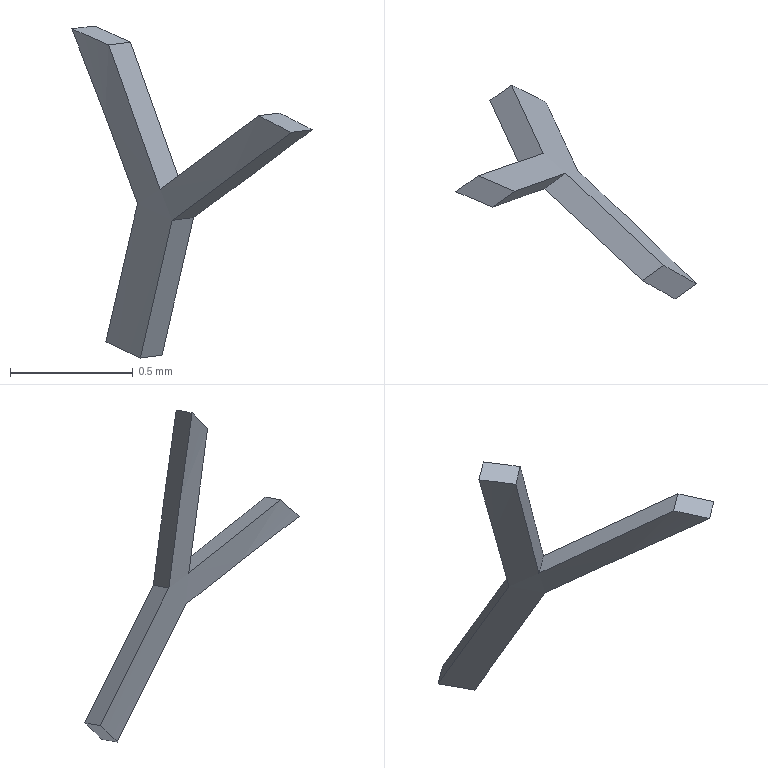Part | SolidWorks | features BaseBody 1 | 1 solid | 11 faces | box 0.9771 x 0.8707 x 1.35 mm | volume 0.03036 mm3 | plane 9 | cylinder 2 | commonest cylinder face diameters 16.8 x1 17 x1
STEP:
#1=CARTESIAN_POINT('',(1971.121,-237.195,995.991));
#2=VERTEX_POINT('',#1);
#3=CARTESIAN_POINT('',(1971.25,-237.473,996.551));
#4=VERTEX_POINT('',#3);
#5=CARTESIAN_POINT('',(1971.931,-238.948,999.517));
#6=DIRECTION('',(0.2015,-0.436,0.8771));
#7=VECTOR('',#6,1000.);
#8=LINE('',#5,#7);
#9=EDGE_CURVE('',#2,#4,#8,.T.);
#10=ORIENTED_EDGE('',*,*,#9,.T.);
#11=CARTESIAN_POINT('',(1971.734,-237.933,996.909));
#12=VERTEX_POINT('',#11);
#13=CARTESIAN_POINT('',(1971.25,-237.473,996.551));
#14=CARTESIAN_POINT('',(1971.414,-237.623,996.67));
#15=CARTESIAN_POINT('',(1971.575,-237.777,996.79));
#16=CARTESIAN_POINT('',(1971.734,-237.933,996.909));
#17=B_SPLINE_CURVE_WITH_KNOTS('',3,(#13,#14,#15,#16),.UNSPECIFIED.,.F.,.F.,(4,4),(0.,1.),.UNSPECIFIED.);
#18=EDGE_CURVE('',#4,#12,#17,.T.);
#19=ORIENTED_EDGE('',*,*,#18,.T.);
#20=CARTESIAN_POINT('',(1971.601,-237.859,996.976));
#21=VERTEX_POINT('',#20);
#22=CARTESIAN_POINT('',(1966.892,-244.458,994.777));
#23=DIRECTION('',(0.2015,-0.436,0.8771));
#24=DIRECTION('',(-0.7309,-0.6631,-0.1618));
#25=AXIS2_PLACEMENT_3D('',#22,#23,#24);
#26=CIRCLE('',#25,8.4);
#27=EDGE_CURVE('',#12,#21,#26,.T.);
#28=ORIENTED_EDGE('',*,*,#27,.T.);
#29=CARTESIAN_POINT('',(1971.201,-237.485,996.678));
#30=VERTEX_POINT('',#29);
#31=CARTESIAN_POINT('',(1971.201,-237.485,996.678));
#32=CARTESIAN_POINT('',(1971.336,-237.607,996.777));
#33=CARTESIAN_POINT('',(1971.47,-237.732,996.877));
#34=CARTESIAN_POINT('',(1971.601,-237.859,996.976));
#35=B_SPLINE_CURVE_WITH_KNOTS('',3,(#31,#32,#33,#34),.UNSPECIFIED.,.F.,.F.,(4,4),(0.,1.),.UNSPECIFIED.);
#36=EDGE_CURVE('',#30,#21,#35,.T.);
#37=ORIENTED_EDGE('',*,*,#36,.F.);
#38=CARTESIAN_POINT('',(1970.991,-237.561,997.264));
#39=VERTEX_POINT('',#38);
#40=CARTESIAN_POINT('',(1970.991,-237.561,997.264));
#41=CARTESIAN_POINT('',(1971.063,-237.534,997.07));
#42=CARTESIAN_POINT('',(1971.133,-237.509,996.874));
#43=CARTESIAN_POINT('',(1971.201,-237.485,996.678));
#44=B_SPLINE_CURVE_WITH_KNOTS('',3,(#40,#41,#42,#43),.UNSPECIFIED.,.F.,.F.,(4,4),(0.,1.),.UNSPECIFIED.);
#45=EDGE_CURVE('',#39,#30,#44,.T.);
#46=ORIENTED_EDGE('',*,*,#45,.F.);
#47=CARTESIAN_POINT('',(1970.842,-237.499,997.33));
#48=VERTEX_POINT('',#47);
#49=CARTESIAN_POINT('',(1966.892,-244.458,994.777));
#50=DIRECTION('',(0.2015,-0.436,0.8771));
#51=DIRECTION('',(-0.7309,-0.6631,-0.1618));
#52=AXIS2_PLACEMENT_3D('',#49,#50,#51);
#53=CIRCLE('',#52,8.4);
#54=EDGE_CURVE('',#39,#48,#53,.T.);
#55=ORIENTED_EDGE('',*,*,#54,.T.);
#56=CARTESIAN_POINT('',(1971.109,-237.404,996.618));
#57=VERTEX_POINT('',#56);
#58=CARTESIAN_POINT('',(1970.842,-237.499,997.33));
#59=CARTESIAN_POINT('',(1970.935,-237.465,997.094));
#60=CARTESIAN_POINT('',(1971.024,-237.433,996.857));
#61=CARTESIAN_POINT('',(1971.109,-237.404,996.618));
#62=B_SPLINE_CURVE_WITH_KNOTS('',3,(#58,#59,#60,#61),.UNSPECIFIED.,.F.,.F.,(4,4),(0.,1.),.UNSPECIFIED.);
#63=EDGE_CURVE('',#48,#57,#62,.T.);
#64=ORIENTED_EDGE('',*,*,#63,.T.);
#65=CARTESIAN_POINT('',(1970.981,-237.126,996.058));
#66=VERTEX_POINT('',#65);
#67=CARTESIAN_POINT('',(1971.79,-238.879,999.584));
#68=DIRECTION('',(-0.2015,0.436,-0.8771));
#69=VECTOR('',#68,1000.);
#70=LINE('',#67,#69);
#71=EDGE_CURVE('',#57,#66,#70,.T.);
#72=ORIENTED_EDGE('',*,*,#71,.T.);
#73=CARTESIAN_POINT('',(1966.64,-243.913,993.681));
#74=DIRECTION('',(-0.2015,0.436,-0.8771));
#75=DIRECTION('',(-0.7309,-0.6631,-0.1618));
#76=AXIS2_PLACEMENT_3D('',#73,#74,#75);
#77=CIRCLE('',#76,8.4);
#78=EDGE_CURVE('',#66,#2,#77,.T.);
#79=ORIENTED_EDGE('',*,*,#78,.T.);
#80=EDGE_LOOP('',(#10,#19,#28,#37,#46,#55,#64,#72,#79));
#81=FACE_OUTER_BOUND('',#80,.T.);
#82=CARTESIAN_POINT('',(1967.45,-245.666,997.207));
#83=DIRECTION('',(0.2015,-0.436,0.8771));
#84=DIRECTION('',(-0.7309,-0.6631,-0.1618));
#85=AXIS2_PLACEMENT_3D('',#82,#83,#84);
#86=CYLINDRICAL_SURFACE('',#85,8.4);
#87=ADVANCED_FACE('',(#81),#86,.F.);
#88=CARTESIAN_POINT('',(1971.209,-237.132,996.003));
#89=VERTEX_POINT('',#88);
#90=CARTESIAN_POINT('',(1971.165,-237.163,995.997));
#91=DIRECTION('',(-0.8088,-0.5792,-0.1022));
#92=VECTOR('',#91,1000.);
#93=LINE('',#90,#92);
#94=EDGE_CURVE('',#89,#2,#93,.T.);
#95=ORIENTED_EDGE('',*,*,#94,.T.);
#96=ORIENTED_EDGE('',*,*,#78,.F.);
#97=CARTESIAN_POINT('',(1971.069,-237.063,996.069));
#98=VERTEX_POINT('',#97);
#99=CARTESIAN_POINT('',(1971.025,-237.094,996.063));
#100=DIRECTION('',(-0.8088,-0.5792,-0.1022));
#101=VECTOR('',#100,1000.);
#102=LINE('',#99,#101);
#103=EDGE_CURVE('',#98,#66,#102,.T.);
#104=ORIENTED_EDGE('',*,*,#103,.F.);
#105=CARTESIAN_POINT('',(1966.64,-243.913,993.681));
#106=DIRECTION('',(-0.2015,0.436,-0.8771));
#107=DIRECTION('',(-0.7309,-0.6631,-0.1618));
#108=AXIS2_PLACEMENT_3D('',#105,#106,#107);
#109=CIRCLE('',#108,8.5);
#110=EDGE_CURVE('',#98,#89,#109,.T.);
#111=ORIENTED_EDGE('',*,*,#110,.T.);
#112=EDGE_LOOP('',(#95,#96,#104,#111));
#113=FACE_OUTER_BOUND('',#112,.T.);
#114=CARTESIAN_POINT('',(1982.308,-239.633,992.21));
#115=DIRECTION('',(-0.2015,0.436,-0.8771));
#116=DIRECTION('',(-0.5526,0.6888,0.4693));
#117=AXIS2_PLACEMENT_3D('',#114,#115,#116);
#118=PLANE('',#117);
#119=ADVANCED_FACE('',(#113),#118,.T.);
#120=ORIENTED_EDGE('',*,*,#103,.T.);
#121=ORIENTED_EDGE('',*,*,#71,.F.);
#122=CARTESIAN_POINT('',(1971.197,-237.341,996.629));
#123=VERTEX_POINT('',#122);
#124=CARTESIAN_POINT('',(1971.153,-237.373,996.623));
#125=DIRECTION('',(-0.8088,-0.5792,-0.1022));
#126=VECTOR('',#125,1000.);
#127=LINE('',#124,#126);
#128=EDGE_CURVE('',#123,#57,#127,.T.);
#129=ORIENTED_EDGE('',*,*,#128,.F.);
#130=CARTESIAN_POINT('',(1971.133,-237.202,996.349));
#131=DIRECTION('',(-0.2015,0.436,-0.8771));
#132=VECTOR('',#131,1000.);
#133=LINE('',#130,#132);
#134=EDGE_CURVE('',#123,#98,#133,.T.);
#135=ORIENTED_EDGE('',*,*,#134,.T.);
#136=EDGE_LOOP('',(#120,#121,#129,#135));
#137=FACE_OUTER_BOUND('',#136,.T.);
#138=CARTESIAN_POINT('',(1977.026,-233.167,997.365));
#139=DIRECTION('',(-0.5526,0.6888,0.4693));
#140=DIRECTION('',(0.2015,-0.436,0.8771));
#141=AXIS2_PLACEMENT_3D('',#138,#139,#140);
#142=PLANE('',#141);
#143=ADVANCED_FACE('',(#137),#142,.T.);
#144=ORIENTED_EDGE('',*,*,#128,.T.);
#145=ORIENTED_EDGE('',*,*,#63,.F.);
#146=CARTESIAN_POINT('',(1970.933,-237.434,997.341));
#147=VERTEX_POINT('',#146);
#148=CARTESIAN_POINT('',(1970.888,-237.466,997.335));
#149=DIRECTION('',(-0.8088,-0.5792,-0.1022));
#150=VECTOR('',#149,1000.);
#151=LINE('',#148,#150);
#152=EDGE_CURVE('',#147,#48,#151,.T.);
#153=ORIENTED_EDGE('',*,*,#152,.F.);
#154=CARTESIAN_POINT('',(1970.933,-237.434,997.341));
#155=CARTESIAN_POINT('',(1970.988,-237.414,997.2));
#156=CARTESIAN_POINT('',(1971.042,-237.394,997.058));
#157=CARTESIAN_POINT('',(1971.095,-237.376,996.915));
#158=CARTESIAN_POINT('',(1971.147,-237.358,996.772));
#159=CARTESIAN_POINT('',(1971.197,-237.341,996.629));
#160=B_SPLINE_CURVE_WITH_KNOTS('',5,(#154,#155,#156,#157,#158,#159),.UNSPECIFIED.,.F.,.F.,(6,6),(0.,1.),.UNSPECIFIED.);
#161=EDGE_CURVE('',#147,#123,#160,.T.);
#162=ORIENTED_EDGE('',*,*,#161,.T.);
#163=EDGE_LOOP('',(#144,#145,#153,#162));
#164=FACE_OUTER_BOUND('',#163,.T.);
#165=CARTESIAN_POINT('',(1976.919,-233.147,998.097));
#166=DIRECTION('',(-0.5701,0.8147,-0.1059));
#167=DIRECTION('',(-0.1446,0.02737,0.9891));
#168=AXIS2_PLACEMENT_3D('',#165,#166,#167);
#169=PLANE('',#168);
#170=ADVANCED_FACE('',(#164),#169,.T.);
#171=ORIENTED_EDGE('',*,*,#152,.T.);
#172=ORIENTED_EDGE('',*,*,#54,.F.);
#173=CARTESIAN_POINT('',(1971.081,-237.497,997.276));
#174=VERTEX_POINT('',#173);
#175=CARTESIAN_POINT('',(1971.036,-237.529,997.27));
#176=DIRECTION('',(-0.8088,-0.5792,-0.1022));
#177=VECTOR('',#176,1000.);
#178=LINE('',#175,#177);
#179=EDGE_CURVE('',#174,#39,#178,.T.);
#180=ORIENTED_EDGE('',*,*,#179,.F.);
#181=CARTESIAN_POINT('',(1966.892,-244.458,994.777));
#182=DIRECTION('',(0.2015,-0.436,0.8771));
#183=DIRECTION('',(-0.7309,-0.6631,-0.1618));
#184=AXIS2_PLACEMENT_3D('',#181,#182,#183);
#185=CIRCLE('',#184,8.5);
#186=EDGE_CURVE('',#174,#147,#185,.T.);
#187=ORIENTED_EDGE('',*,*,#186,.T.);
#188=EDGE_LOOP('',(#171,#172,#180,#187));
#189=FACE_OUTER_BOUND('',#188,.T.);
#190=CARTESIAN_POINT('',(1982.415,-239.999,993.428));
#191=DIRECTION('',(0.2015,-0.436,0.8771));
#192=DIRECTION('',(0.5526,-0.6888,-0.4693));
#193=AXIS2_PLACEMENT_3D('',#190,#191,#192);
#194=PLANE('',#193);
#195=ADVANCED_FACE('',(#189),#194,.T.);
#196=ORIENTED_EDGE('',*,*,#179,.T.);
#197=ORIENTED_EDGE('',*,*,#45,.T.);
#198=CARTESIAN_POINT('',(1971.289,-237.422,996.689));
#199=VERTEX_POINT('',#198);
#200=CARTESIAN_POINT('',(1971.245,-237.453,996.683));
#201=DIRECTION('',(-0.8088,-0.5792,-0.1022));
#202=VECTOR('',#201,1000.);
#203=LINE('',#200,#202);
#204=EDGE_CURVE('',#199,#30,#203,.T.);
#205=ORIENTED_EDGE('',*,*,#204,.F.);
#206=CARTESIAN_POINT('',(1971.081,-237.497,997.276));
#207=CARTESIAN_POINT('',(1971.124,-237.481,997.159));
#208=CARTESIAN_POINT('',(1971.166,-237.465,997.042));
#209=CARTESIAN_POINT('',(1971.208,-237.45,996.924));
#210=CARTESIAN_POINT('',(1971.249,-237.436,996.807));
#211=CARTESIAN_POINT('',(1971.289,-237.422,996.689));
#212=B_SPLINE_CURVE_WITH_KNOTS('',5,(#206,#207,#208,#209,#210,#211),.UNSPECIFIED.,.F.,.F.,(6,6),(0.,1.),.UNSPECIFIED.);
#213=EDGE_CURVE('',#174,#199,#212,.T.);
#214=ORIENTED_EDGE('',*,*,#213,.F.);
#215=EDGE_LOOP('',(#196,#197,#205,#214));
#216=FACE_OUTER_BOUND('',#215,.T.);
#217=CARTESIAN_POINT('',(1977.09,-233.267,997.422));
#218=DIRECTION('',(0.5712,-0.8149,0.09826));
#219=DIRECTION('',(0.1402,-0.0211,-0.9899));
#220=AXIS2_PLACEMENT_3D('',#217,#218,#219);
#221=PLANE('',#220);
#222=ADVANCED_FACE('',(#216),#221,.T.);
#223=ORIENTED_EDGE('',*,*,#204,.T.);
#224=ORIENTED_EDGE('',*,*,#36,.T.);
#225=CARTESIAN_POINT('',(1971.687,-237.797,996.987));
#226=VERTEX_POINT('',#225);
#227=CARTESIAN_POINT('',(1971.644,-237.828,996.982));
#228=DIRECTION('',(-0.8088,-0.5792,-0.1022));
#229=VECTOR('',#228,1000.);
#230=LINE('',#227,#229);
#231=EDGE_CURVE('',#226,#21,#230,.T.);
#232=ORIENTED_EDGE('',*,*,#231,.F.);
#233=CARTESIAN_POINT('',(1971.289,-237.422,996.689));
#234=CARTESIAN_POINT('',(1971.37,-237.496,996.749));
#235=CARTESIAN_POINT('',(1971.45,-237.57,996.808));
#236=CARTESIAN_POINT('',(1971.53,-237.645,996.868));
#237=CARTESIAN_POINT('',(1971.609,-237.721,996.927));
#238=CARTESIAN_POINT('',(1971.687,-237.797,996.987));
#239=B_SPLINE_CURVE_WITH_KNOTS('',5,(#233,#234,#235,#236,#237,#238),.UNSPECIFIED.,.F.,.F.,(6,6),(0.,1.),.UNSPECIFIED.);
#240=EDGE_CURVE('',#199,#226,#239,.T.);
#241=ORIENTED_EDGE('',*,*,#240,.F.);
#242=EDGE_LOOP('',(#223,#224,#232,#241));
#243=FACE_OUTER_BOUND('',#242,.T.);
#244=CARTESIAN_POINT('',(1977.379,-233.721,997.706));
#245=DIRECTION('',(-0.3469,0.3295,0.8781));
#246=DIRECTION('',(0.4749,-0.7456,0.4674));
#247=AXIS2_PLACEMENT_3D('',#244,#245,#246);
#248=PLANE('',#247);
#249=ADVANCED_FACE('',(#243),#248,.T.);
#250=ORIENTED_EDGE('',*,*,#231,.T.);
#251=ORIENTED_EDGE('',*,*,#27,.F.);
#252=CARTESIAN_POINT('',(1971.819,-237.872,996.92));
#253=VERTEX_POINT('',#252);
#254=CARTESIAN_POINT('',(1971.776,-237.903,996.914));
#255=DIRECTION('',(-0.8088,-0.5792,-0.1022));
#256=VECTOR('',#255,1000.);
#257=LINE('',#254,#256);
#258=EDGE_CURVE('',#253,#12,#257,.T.);
#259=ORIENTED_EDGE('',*,*,#258,.F.);
#260=CARTESIAN_POINT('',(1966.892,-244.458,994.777));
#261=DIRECTION('',(0.2015,-0.436,0.8771));
#262=DIRECTION('',(-0.7309,-0.6631,-0.1618));
#263=AXIS2_PLACEMENT_3D('',#260,#261,#262);
#264=CIRCLE('',#263,8.5);
#265=EDGE_CURVE('',#253,#226,#264,.T.);
#266=ORIENTED_EDGE('',*,*,#265,.T.);
#267=EDGE_LOOP('',(#250,#251,#259,#266));
#268=FACE_OUTER_BOUND('',#267,.T.);
#269=CARTESIAN_POINT('',(1982.415,-239.999,993.428));
#270=DIRECTION('',(0.2015,-0.436,0.8771));
#271=DIRECTION('',(0.5526,-0.6888,-0.4693));
#272=AXIS2_PLACEMENT_3D('',#269,#270,#271);
#273=PLANE('',#272);
#274=ADVANCED_FACE('',(#268),#273,.T.);
#275=ORIENTED_EDGE('',*,*,#258,.T.);
#276=ORIENTED_EDGE('',*,*,#18,.F.);
#277=CARTESIAN_POINT('',(1971.337,-237.41,996.562));
#278=VERTEX_POINT('',#277);
#279=CARTESIAN_POINT('',(1971.294,-237.442,996.557));
#280=DIRECTION('',(-0.8088,-0.5792,-0.1022));
#281=VECTOR('',#280,1000.);
#282=LINE('',#279,#281);
#283=EDGE_CURVE('',#278,#4,#282,.T.);
#284=ORIENTED_EDGE('',*,*,#283,.F.);
#285=CARTESIAN_POINT('',(1971.337,-237.41,996.562));
#286=CARTESIAN_POINT('',(1971.435,-237.501,996.634));
#287=CARTESIAN_POINT('',(1971.533,-237.592,996.705));
#288=CARTESIAN_POINT('',(1971.629,-237.685,996.777));
#289=CARTESIAN_POINT('',(1971.725,-237.778,996.848));
#290=CARTESIAN_POINT('',(1971.819,-237.872,996.92));
#291=B_SPLINE_CURVE_WITH_KNOTS('',5,(#285,#286,#287,#288,#289,#290),.UNSPECIFIED.,.F.,.F.,(6,6),(0.,1.),.UNSPECIFIED.);
#292=EDGE_CURVE('',#278,#253,#291,.T.);
#293=ORIENTED_EDGE('',*,*,#292,.T.);
#294=EDGE_LOOP('',(#275,#276,#284,#293));
#295=FACE_OUTER_BOUND('',#294,.T.);
#296=CARTESIAN_POINT('',(1977.112,-233.275,997.292));
#297=DIRECTION('',(0.3433,-0.3238,-0.8817));
#298=DIRECTION('',(-0.4776,0.7481,-0.4607));
#299=AXIS2_PLACEMENT_3D('',#296,#297,#298);
#300=PLANE('',#299);
#301=ADVANCED_FACE('',(#295),#300,.T.);
#302=ORIENTED_EDGE('',*,*,#283,.T.);
#303=ORIENTED_EDGE('',*,*,#9,.F.);
#304=ORIENTED_EDGE('',*,*,#94,.F.);
#305=CARTESIAN_POINT('',(1971.273,-237.271,996.282));
#306=DIRECTION('',(0.2015,-0.436,0.8771));
#307=VECTOR('',#306,1000.);
#308=LINE('',#305,#307);
#309=EDGE_CURVE('',#89,#278,#308,.T.);
#310=ORIENTED_EDGE('',*,*,#309,.T.);
#311=EDGE_LOOP('',(#302,#303,#304,#310));
#312=FACE_OUTER_BOUND('',#311,.T.);
#313=CARTESIAN_POINT('',(1976.983,-232.996,996.732));
#314=DIRECTION('',(0.5526,-0.6888,-0.4693));
#315=DIRECTION('',(-0.2015,0.436,-0.8771));
#316=AXIS2_PLACEMENT_3D('',#313,#314,#315);
#317=PLANE('',#316);
#318=ADVANCED_FACE('',(#312),#317,.T.);
#319=ORIENTED_EDGE('',*,*,#110,.F.);
#320=ORIENTED_EDGE('',*,*,#134,.F.);
#321=ORIENTED_EDGE('',*,*,#161,.F.);
#322=ORIENTED_EDGE('',*,*,#186,.F.);
#323=ORIENTED_EDGE('',*,*,#213,.T.);
#324=ORIENTED_EDGE('',*,*,#240,.T.);
#325=ORIENTED_EDGE('',*,*,#265,.F.);
#326=ORIENTED_EDGE('',*,*,#292,.F.);
#327=ORIENTED_EDGE('',*,*,#309,.F.);
#328=EDGE_LOOP('',(#319,#320,#321,#322,#323,#324,#325,#326,#327));
#329=FACE_OUTER_BOUND('',#328,.T.);
#330=CARTESIAN_POINT('',(1967.45,-245.666,997.207));
#331=DIRECTION('',(0.2015,-0.436,0.8771));
#332=DIRECTION('',(-0.7309,-0.6631,-0.1618));
#333=AXIS2_PLACEMENT_3D('',#330,#331,#332);
#334=CYLINDRICAL_SURFACE('',#333,8.5);
#335=ADVANCED_FACE('',(#329),#334,.T.);
#336=CLOSED_SHELL('',(#87,#119,#143,#170,#195,#222,#249,#274,#301,#318,#335));
#337=MANIFOLD_SOLID_BREP('',#336);
#338=CARTESIAN_POINT('',(0.,0.,0.));
#339=DIRECTION('',(0.,0.,1.));
#340=DIRECTION('',(1.,0.,0.));
#341=AXIS2_PLACEMENT_3D('',#338,#339,#340);
#342=(LENGTH_UNIT()NAMED_UNIT(*)SI_UNIT(.MILLI.,.METRE.));
#343=UNCERTAINTY_MEASURE_WITH_UNIT(LENGTH_MEASURE(0.00001),#342,'','');
#344=(NAMED_UNIT(*)PLANE_ANGLE_UNIT()SI_UNIT($,.RADIAN.));
#345=(NAMED_UNIT(*)SI_UNIT($,.STERADIAN.)SOLID_ANGLE_UNIT());
#346=(GEOMETRIC_REPRESENTATION_CONTEXT(3)GLOBAL_UNCERTAINTY_ASSIGNED_CONTEXT((#343))GLOBAL_UNIT_ASSIGNED_CONTEXT((#342,#344,#345))REPRESENTATION_CONTEXT('',''));
#347=ADVANCED_BREP_SHAPE_REPRESENTATION('',(#337,#341),#346);